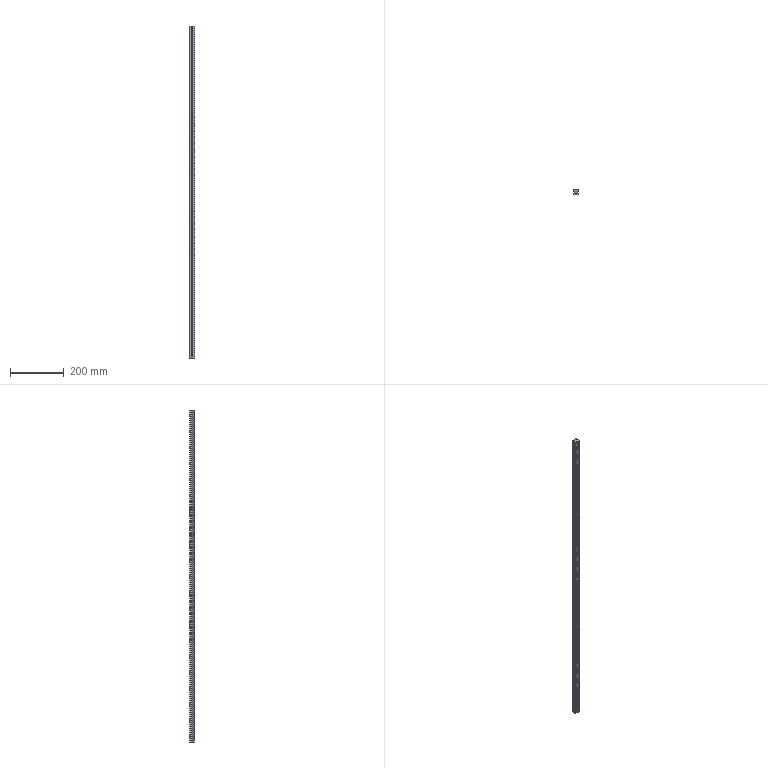Part | SolidWorks | features BaseBody 1 | 1 solid | 198 faces | box 20 x 18 x 1240 mm | volume 355945 mm3 | plane 110 | cylinder 88 | commonest cylinder face diameters 6 x42 9.5 x42 4.12 x4